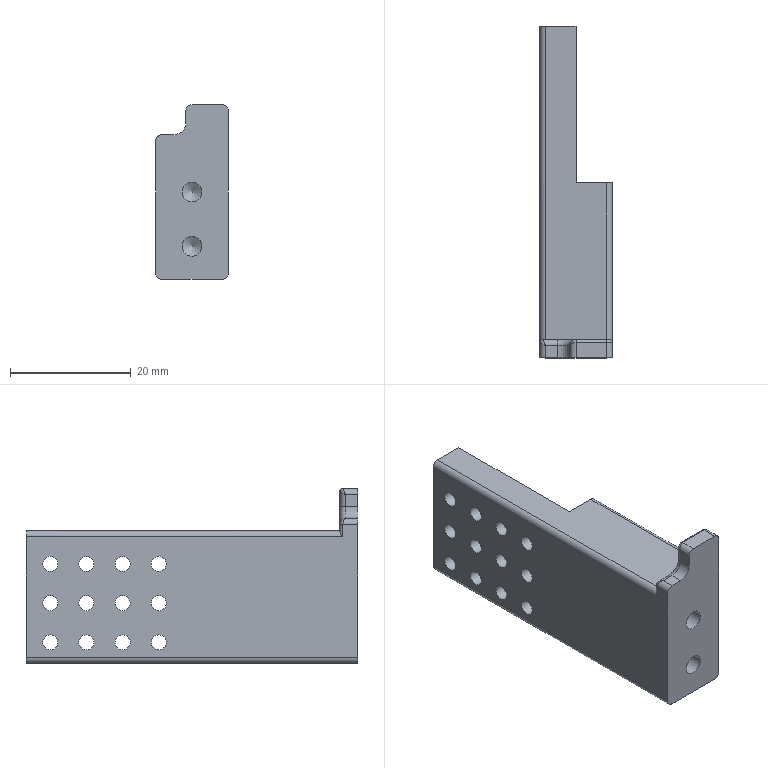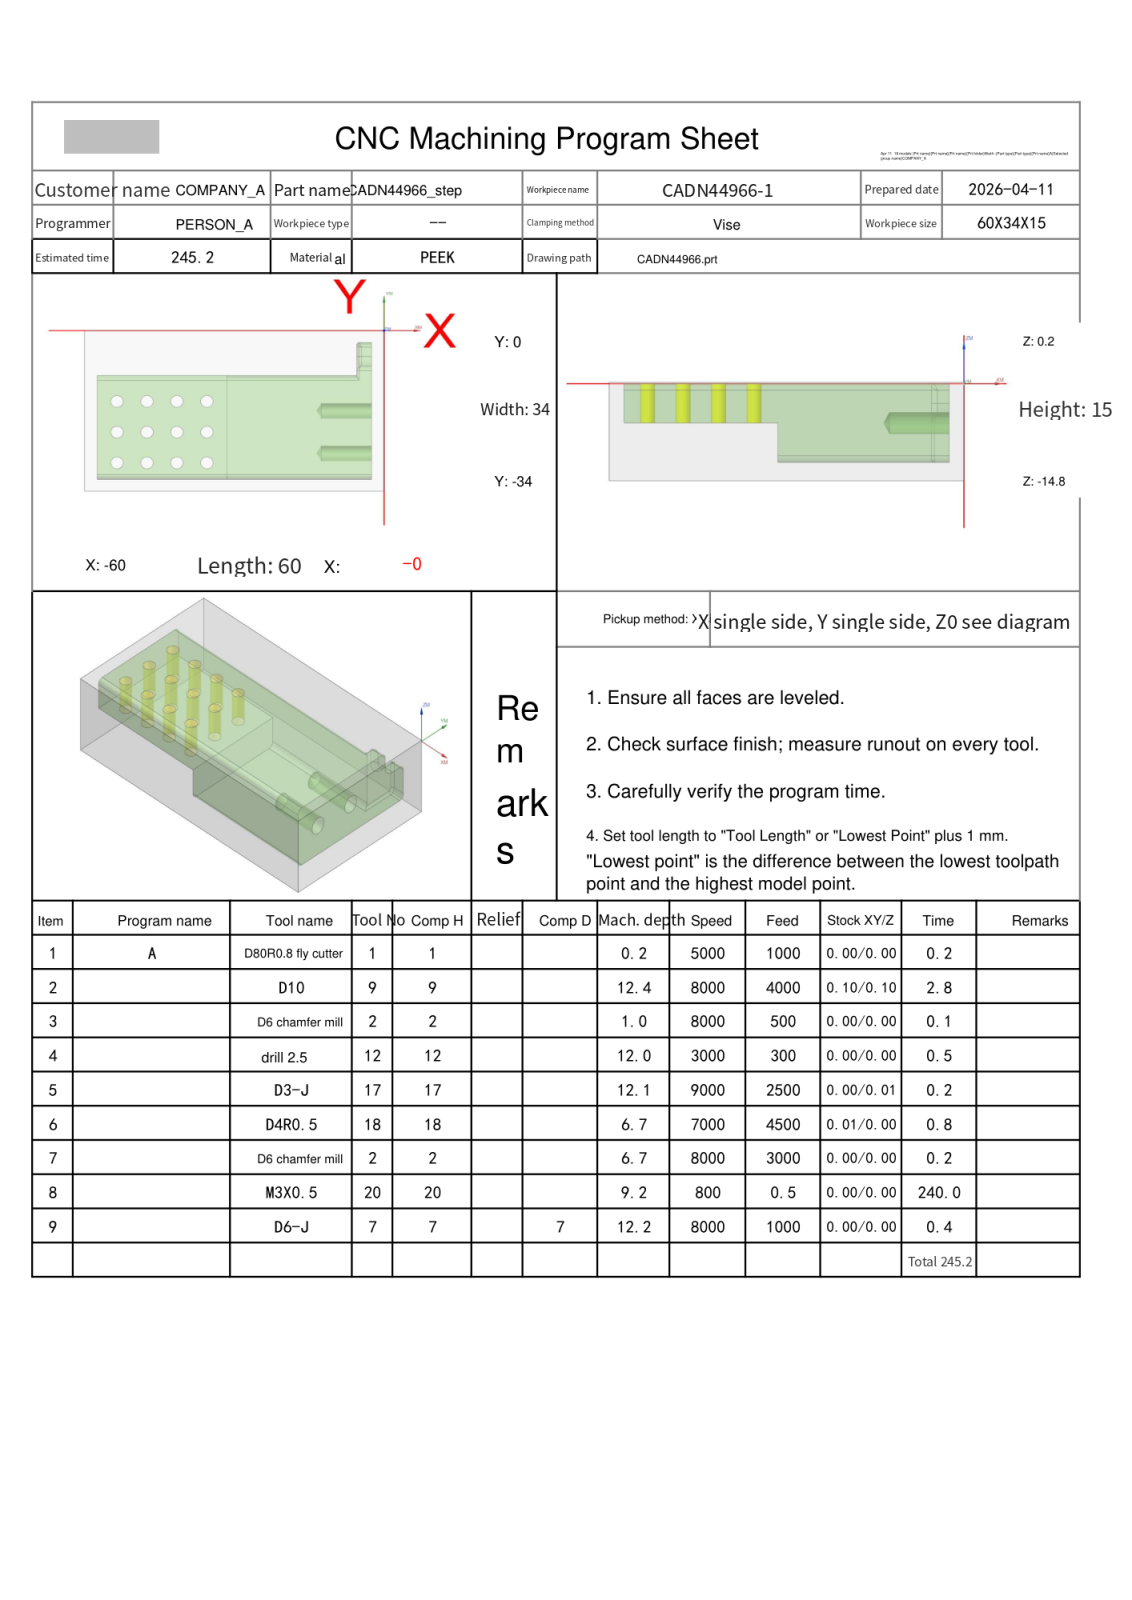NC program | NX | posted by the shop | part box 12 x 55 x 29 mm
Lines 2145 to 3281 of 3281:
N6 T18 M06
(D4R0.5  D=4. R=0.5 H=18 ce=0.01 di=0.00)
G00 G90 G54 X1.72 Y-32.322 M03 S7000
G43 H18 Z10.2
M08
Z.488
G01 Z-.012 F4500.
X-1.4 Y-32.113
G03 X-1.655 Y-32.105 I-.255 J-3.807
X-2.5 Y-32.199 I0.0 J-3.816
G01 X-57.5
X-58.6 Y-32.111
Y-32.156 Z-.02
Y-32.174 Z-.028
X-57.5 Y-32.3
X-2.5
G02 X-1.584 Y-32.179 I.916 J-3.411
G01 X-1.4 Y-32.184
Y-32.251 Z-.038
Y-32.268 Z-.048
X-2.5 Y-32.385
X-57.5
X-58.6 Y-32.25
Y-32.307 Z-.059
Y-32.338 Z-.07
X-57.5 Y-32.463
X-2.5
G02 X-1.42 Y-32.365 I1.08 J-5.877
G01 X-1.4
Y-32.407 Z-.084
Y-32.429 Z-.097
G03 X-2.5 Y-32.541 I.01 J-5.57
G01 X-57.5
G03 X-58.6 Y-32.415 I-1.468 J-7.964
G01 Y-32.465 Z-.113
Y-32.494 Z-.13
G02 X-57.5 Y-32.62 I-.279 J-7.329
G01 X-2.5
G02 X-1.4 Y-32.505 I1.119 J-5.41
G01 Y-32.56 Z-.149
Y-32.595 Z-.168
G03 X-2.5 Y-32.7 I.124 J-7.151
G01 X-57.5
G03 X-58.6 Y-32.588 I-1.463 J-8.959
G01 Y-32.643 Z-.19
Y-32.685 Z-.212
G02 X-57.5 Y-32.779 I-.1 J-7.651
G01 X-2.5
G02 X-1.4 Y-32.688 I1.138 J-7.013
G01 X-1.399 Y-32.734 Z-.237
X-1.398 Y-32.78 Z-.263
X-1.405
G03 X-2.5 Y-32.858 I0.0 J-7.705
G01 X-57.5
G03 X-58.593 Y-32.78 I-1.093 J-7.602
G01 X-58.602
Y-32.818 Z-.291
X-58.601 Y-32.855 Z-.319
X-58.583
G02 X-57.5 Y-32.935 I0.0 J-7.43
G01 X-2.5
G02 X-1.411 Y-32.855 I1.089 J-7.418
G01 X-1.399
X-1.4 Y-32.895 Z-.35
Y-32.934 Z-.38
X-1.45
G03 X-2.5 Y-33.008 I0.0 J-7.494
G01 X-57.5
G03 X-58.547 Y-32.934 I-1.047 J-7.396
G01 X-58.6
X-58.601 Y-32.979 Z-.414
Y-33.012 Z-.447
X-58.596
G02 X-57.5 Y-33.078 I0.0 J-9.139
G01 X-2.5
G02 X-1.401 Y-33.012 I1.099 J-9.111
G01 X-1.399
Y-33.05 Z-.483
Y-33.086 Z-.519
X-1.502 Y-33.085
G03 X-2.5 Y-33.145 I0.0 J-8.383
G01 X-57.5
G03 X-58.494 Y-33.085 I-.994 J-8.274
G01 X-58.602 Y-33.086
X-58.601 Y-33.116 Z-.557
Y-33.145 Z-.596
X-58.517
G02 X-57.5 Y-33.207 I0.0 J-8.403
G01 X-2.5
G02 X-1.48 Y-33.145 I1.02 J-8.367
G01 X-1.399
X-1.4 Y-33.177 Z-.636
Y-33.207 Z-.676
X-1.518
G03 X-2.5 Y-33.264 I0.0 J-8.497
G01 X-57.5
G03 X-58.444 Y-33.206 I-.944 J-7.719
G01 X-58.6 Y-33.208
X-58.601 Y-33.24 Z-.718
X-58.602 Y-33.267 Z-.761
X-58.472 Y-33.266
G02 X-57.5 Y-33.315 I0.0 J-9.699
G01 X-2.5
G02 X-1.52 Y-33.266 I.979 J-9.79
G01 X-1.398 Y-33.267
Y-33.287 Z-.805
Y-33.31 Z-.849
X-1.444
G03 X-2.5 Y-33.361 I0.0 J-10.853
G01 X-57.5
G03 X-58.486 Y-33.312 I-.986 J-9.766
G01 X-58.602
Y-33.335 Z-.894
Y-33.356 Z-.94
X-58.424 Y-33.354
G02 X-57.5 Y-33.401 I0.0 J-9.019
G01 X-2.5
G02 X-1.429 Y-33.35 I1.071 J-11.207
G01 X-1.398
Y-33.371 Z-.987
Y-33.39 Z-1.034
G03 X-2.5 Y-33.436 I.189 J-17.771
G01 X-57.5
G03 X-58.404 Y-33.397 I-.904 J-10.532
G01 X-58.603 Y-33.399
X-58.602 Y-33.415 Z-1.081
Y-33.432 Z-1.129
X-58.426 Y-33.431
G02 X-57.5 Y-33.464 I0.0 J-13.202
G01 X-2.5
G02 X-1.398 Y-33.425 I1.263 J-20.561
G01 X-1.399 Y-33.442 Z-1.176
Y-33.453 Z-1.222
G03 X-2.5 Y-33.484 I.082 J-22.15
G01 X-57.5
G03 X-58.395 Y-33.457 I-.895 J-14.646
X-58.601 Y-33.458 I0.0 J-14.674
G01 X-58.6 Y-33.476 Z-1.268
Y-33.484 Z-1.315
G02 X-58.344 Y-33.483 I.256 J-22.307
X-57.5 Y-33.499 I0.0 J-22.309
G01 X-2.5
X-1.4 Y-33.48
Y-33.491 Z-1.361
Y-33.498 Z-1.407
X-2.5 Y-33.507
X-57.5
X-58.602 Y-33.499
Y-33.508 Z-1.454
X-58.603 Y-33.51 Z-1.5
X-1.4
G00 Z10.2
G00 G90 X-61.837 Y-8.898 M03 S7000
Z10.2
Z.488
G01 Z-.012 F4500.
X-58.603 Y-8.894
X-57.5 Y-8.802
X-6.663
Y-8.5
Y-8.485
G02 X-4.996 Y-6.802 I1.682 J0.0
G01 X-2.5
X-1.4 Y-6.883
Y-6.848 Z-.019
Y-6.83 Z-.026
X-1.411
G02 X-2.5 Y-6.712 I0.0 J5.057
G01 X-4.991
G03 X-6.737 Y-8.479 I.021 J-1.767
G01 Y-8.5
Y-8.712
X-57.5
G02 X-58.316 Y-8.821 I-.816 J2.98
X-58.601 Y-8.808 I0.0 J3.09
G01 X-58.603 Y-8.767 Z-.034
X-58.605 Y-8.726 Z-.043
G03 X-58.274 Y-8.747 I.331 J2.693
X-57.5 Y-8.634 I0.0 J2.714
G01 X-6.8
Y-8.5
Y-8.474
G02 X-4.985 Y-6.634 I1.84 J0.0
G01 X-2.5
X-1.4 Y-6.768
Y-6.71 Z-.054
Y-6.689 Z-.064
X-2.5 Y-6.556
X-4.978
G03 X-6.863 Y-8.47 I.03 J-1.914
G01 X-6.862 Y-8.5
Y-8.556
X-57.5
G02 X-58.43 Y-8.658 I-.93 J4.19
G01 X-58.602 Y-8.655
X-58.601 Y-8.612 Z-.077
X-58.6 Y-8.573 Z-.09
X-58.552 Y-8.574
G03 X-57.5 Y-8.479 I0.0 J5.897
G01 X-6.923
G02 X-4.969 Y-6.479 I2.016 J-.015
G01 X-2.5
X-1.4 Y-6.599
Y-6.56 Z-.105
Y-6.524 Z-.121
G02 X-2.5 Y-6.4 I.299 J7.568
G01 X-4.959
G03 X-6.926 Y-8.015 I.052 J-2.067
G01 X-6.981 Y-8.4
X-57.5
G02 X-58.6 Y-8.505 I-1.107 J5.765
G01 Y-8.46 Z-.139
Y-8.424 Z-.158
G03 X-57.5 Y-8.32 I-.041 J6.28
G01 X-7.038
G02 X-4.947 Y-6.32 I2.144 J-.149
G01 X-2.5
G03 X-1.4 Y-6.435 I1.366 J7.711
G01 Y-6.382 Z-.18
Y-6.332 Z-.201
G02 X-2.5 Y-6.24 I.09 J7.674
G01 X-4.933
G03 X-7.092 Y-8.24 I.063 J-2.233
G01 X-57.5
G02 X-58.6 Y-8.33 I-1.264 J8.632
G01 Y-8.284 Z-.225
Y-8.25 Z-.25
G03 X-57.5 Y-8.161 I-.001 J6.861
G01 X-7.142
G02 X-4.916 Y-6.161 I2.28 J-.299
G01 X-2.5
G03 X-1.399 Y-6.249 I1.165 J7.674
G01 Y-6.202 Z-.277
Y-6.163 Z-.305
X-1.434 Y-6.164
G02 X-2.5 Y-6.084 I0.0 J7.173
G01 X-4.898
G03 X-7.184 Y-8.073 I.051 J-2.366
G01 X-7.201 Y-8.084
X-57.5
G02 X-58.6 Y-8.174 I-1.183 J7.718
G01 Y-8.124 Z-.335
Y-8.09 Z-.365
G03 X-57.5 Y-8.01 I-.047 J8.233
G01 X-7.231
G02 X-4.878 Y-6.01 I2.407 J-.448
G01 X-2.5
G03 X-1.4 Y-6.085 I1.142 J8.595
G01 Y-6.042 Z-.398
X-1.399 Y-6.001 Z-.43
X-1.432
G02 X-2.5 Y-5.938 I0.0 J9.084
G01 X-4.856
G03 X-7.265 Y-7.938 I.05 J-2.511
G01 X-57.5
G02 X-58.536 Y-8.002 I-1.036 J8.448
G01 X-58.6 Y-8.001
X-58.601 Y-7.96 Z-.466
Y-7.929 Z-.501
X-58.519
G03 X-57.5 Y-7.871 I0.0 J8.943
G01 X-7.296
G02 X-5.641 Y-6.012 I2.54 J-.596
X-4.833 Y-5.871 I.808 J-2.242
G01 X-2.5
G03 X-1.461 Y-5.931 I1.039 J8.991
G01 X-1.399
Y-5.899 Z-.539
Y-5.869 Z-.576
X-1.505 Y-5.87
G02 X-2.5 Y-5.808 I0.0 J8.056
G01 X-4.808
G03 X-7.321 Y-7.81 I.047 J-2.637
G01 X-7.333 Y-7.808
X-57.5
G02 X-58.492 Y-7.87 I-.992 J7.94
G01 X-58.601 Y-7.869
Y-7.838 Z-.616
Y-7.809 Z-.656
X-58.502 Y-7.81
G03 X-57.5 Y-7.75 I0.0 J8.419
G01 X-7.347
G02 X-5.68 Y-5.915 I2.647 J-.73
X-4.781 Y-5.75 I.999 J-2.915
G01 X-2.5
G03 X-1.4 Y-5.808 I1.131 J10.987
G01 Y-5.775 Z-.698
Y-5.75 Z-.74
X-1.445
G02 X-2.5 Y-5.697 I0.0 J10.496
G01 X-4.753
X-4.802 Y-5.704
X-5.085 Y-5.72
G03 X-7.357 Y-7.697 I.382 J-2.734
G01 X-57.5
G02 X-58.519 Y-7.747 I-1.019 J10.41
G01 X-58.6 Y-7.746
Y-7.725 Z-.783
Y-7.701 Z-.827
X-58.462 Y-7.702
G03 X-57.5 Y-7.649 I0.0 J8.811
G01 X-7.367
G02 X-6.217 Y-6.104 I2.749 J-.845
X-4.724 Y-5.649 I1.543 J-2.386
G01 X-2.5
G03 X-1.4 Y-5.705 I1.116 J11.228
G01 Y-5.676 Z-.872
Y-5.658 Z-.917
X-1.453
G02 X-2.5 Y-5.608 I0.0 J10.934
G01 X-4.694
G03 X-7.367 Y-7.608 I.039 J-2.838
G01 X-57.5
G02 X-58.589 Y-7.661 I-1.089 J11.136
G01 X-58.6
Y-7.639 Z-.964
Y-7.619 Z-1.011
G03 X-57.5 Y-7.572 I-.112 J15.527
G01 X-7.364
G02 X-4.663 Y-5.572 I2.742 J-.879
G01 X-2.5
G03 X-1.584 Y-5.615 I.916 J9.853
G01 X-1.4 Y-5.613
X-1.399 Y-5.59 Z-1.058
X-1.398 Y-5.576 Z-1.106
X-1.578 Y-5.578
G02 X-2.5 Y-5.543 I0.0 J12.213
G01 X-4.631
G03 X-7.354 Y-7.543 I.039 J-2.907
G01 X-57.5
G02 X-58.599 Y-7.581 I-1.206 J18.777
G01 X-58.6 Y-7.564 Z-1.155
Y-7.548 Z-1.203
G03 X-57.5 Y-7.52 I-.149 J26.922
G01 X-7.346
G02 X-4.599 Y-5.52 I2.789 J-.945
G01 X-2.5
G03 X-1.615 Y-5.545 I.885 J15.399
X-1.396 Y-5.544 I0.0 J15.425
G01 X-1.395 Y-5.535 Z-1.253
X-1.394 Y-5.519 Z-1.302
G02 X-1.646 Y-5.521 I-.252 J20.394
X-2.5 Y-5.503 I0.0 J20.395
G01 X-4.566
X-4.607 Y-5.51
G03 X-5.753 Y-5.763 I.025 J-2.833
X-7.339 Y-7.503 I1.264 J-2.745
G01 X-57.5
G02 X-58.601 Y-7.523 I-1.11 J30.954
G01 X-58.602 Y-7.515 Z-1.352
Y-7.505 Z-1.401
X-57.5 Y-7.493
X-7.335
G02 X-4.677 Y-5.493 I2.841 J-1.009
G01 X-2.5
G03 X-1.649 Y-5.504 I.851 J33.099
G01 X-1.395 Y-5.503
Y-5.494 Z-1.451
Y-5.491 Z-1.5
X-2.5 Y-5.49
X-4.646
G03 X-7.335 Y-7.49 I.158 J-3.021
G01 X-7.491
X-57.5
X-58.603
G00 Z10.2
G00 G90 X-8.666 Y-6.802 M03 S7000
Z10.2
Z.488
G01 Z-.012 F4500.
G03 X-6.666 Y-8.802 I2. J0.0
G01 X-6.675 Y-8.619
G02 X-4.996 Y-6.802 I1.822 J0.0
G01 X-2.5
X-1.399 Y-6.901
Y-6.848 Z-.019
Y-6.826 Z-.026
X-1.526 Y-6.828
G02 X-2.5 Y-6.712 I0.0 J4.152
G01 X-4.991
G03 X-6.747 Y-8.545 I.079 J-1.833
G01 X-6.739 Y-8.712
X-6.757
Y-8.683 Z-.032
X-6.768 Y-8.657 Z-.037
X-6.803 Y-8.633 Z-.043
X-6.806 Y-8.522
G02 X-4.985 Y-6.633 I1.89 J0.0
G01 X-2.5
G03 X-1.399 Y-6.764 I1.139 J4.875
G01 Y-6.712 Z-.054
Y-6.691 Z-.064
G02 X-2.5 Y-6.555 I.5 J8.593
G01 X-4.978
G03 X-6.866 Y-8.519 I.077 J-1.963
G01 Y-8.555
X-6.881
X-6.885 Y-8.523 Z-.073
X-6.892 Y-8.501 Z-.082
X-6.928 Y-8.477 Z-.091
G02 X-4.969 Y-6.477 I2.023 J-.022
G01 X-2.5
G03 X-1.4 Y-6.602 I1.619 J9.345
G01 Y-6.56 Z-.106
Y-6.519 Z-.122
G02 X-2.5 Y-6.397 I.201 J6.798
G01 X-4.959
G03 X-6.985 Y-8.397 I.064 J-2.091
G01 X-6.999
X-6.998 Y-8.368 Z-.135
X-7.021 Y-8.331 Z-.148
X-7.042 Y-8.315 Z-.16
G02 X-4.946 Y-6.315 I2.164 J-.169
G01 X-2.5
G03 X-1.4 Y-6.43 I1.188 J6.081
G01 Y-6.377 Z-.182
Y-6.326 Z-.204
X-1.439
G02 X-2.5 Y-6.235 I0.0 J6.189
G01 X-4.932
G03 X-7.095 Y-8.235 I.056 J-2.23
G01 X-7.146 Y-8.156 Z-.254
G02 X-4.915 Y-6.156 I2.304 J-.325
G01 X-2.5
G02 X-1.924 Y-6.244 I-.064 J-2.338
G01 X-1.4 Y-6.245
Y-6.196 Z-.281
Y-6.168 Z-.309
X-1.924 Y-6.167
G03 X-2.5 Y-6.078 I-.671 J-2.44
G01 X-4.897
G03 X-7.186 Y-8.066 I.049 J-2.368
G01 X-7.203 Y-8.078
X-7.233 Y-8.004 Z-.37
G02 X-4.877 Y-6.004 I2.415 J-.457
G01 X-2.5
G02 X-1.924 Y-6.082 I-.122 J-3.048
G01 X-1.4 Y-6.083
Y-6.036 Z-.403
Y-5.996 Z-.436
X-1.573 Y-5.998
G02 X-2.5 Y-5.933 I0.0 J6.632
G01 X-4.855
G03 X-7.268 Y-7.933 I.048 J-2.513
G01 X-7.299 Y-7.866 Z-.507
G02 X-4.831 Y-5.866 I2.517 J-.583
G01 X-2.5
G03 X-1.561 Y-5.926 I.938 J7.256
G01 X-1.4 Y-5.924
Y-5.894 Z-.545
Y-5.865 Z-.583
X-1.576 Y-5.867
G02 X-2.5 Y-5.803 I0.0 J6.74
G01 X-4.806
G03 X-5.81 Y-6.017 I.083 J-2.859
X-7.327 Y-7.803 I1.093 J-2.464
G01 X-7.343 Y-7.745 Z-.663
G02 X-4.779 Y-5.745 I2.607 J-.699
G01 X-2.5
G03 X-1.574 Y-5.806 I.926 J7.011
G01 X-1.4 Y-5.804
Y-5.773 Z-.705
Y-5.741 Z-.747
X-1.579 Y-5.743
G02 X-2.5 Y-5.693 I0.0 J8.504
G01 X-4.751
G03 X-7.358 Y-7.693 I.043 J-2.755
G01 X-7.366 Y-7.646 Z-.834
G02 X-4.721 Y-5.646 I2.686 J-.803
G01 X-2.5
X-1.924 Y-5.697
X-1.4
X-1.401 Y-5.672 Z-.88
Y-5.653 Z-.925
G02 X-1.623 Y-5.656 I-.222 J7.508
X-2.5 Y-5.605 I0.0 J7.511
G01 X-4.692
G03 X-7.004 Y-6.86 I.031 J-2.814
X-7.365 Y-7.605 I2.346 J-1.596
G01 X-7.385 Y-7.569 Z-1.018
X-7.359 Y-7.559
X-7.332 Y-7.482
G02 X-4.66 Y-5.569 I2.711 J-.966
G01 X-2.5
G03 X-1.662 Y-5.612 I.838 J8.316
X-1.402 Y-5.607 I0.0 J8.359
G01 Y-5.59 Z-1.066
Y-5.572 Z-1.114
G02 X-1.711 Y-5.578 I-.309 J8.411
X-2.5 Y-5.541 I0.0 J8.416
G01 X-4.629
X-4.815 Y-5.553
G03 X-6.774 Y-6.528 I.191 J-2.839
X-7.353 Y-7.541 I2.274 J-1.972
G01 X-7.345 Y-7.518 Z-1.211
G02 X-6.253 Y-6.053 I2.845 J-.982
X-4.63 Y-5.524 I1.657 J-2.327
G01 X-4.596 Y-5.518
X-2.5
G03 X-1.726 Y-5.546 I.774 J10.621
X-1.402 Y-5.541 I0.0 J10.65
G01 X-1.4 Y-5.525 Z-1.261
X-1.399 Y-5.521 Z-1.31
G02 X-1.613 Y-5.522 I-.214 J19.642
X-2.5 Y-5.502 I0.0 J19.643
G01 X-4.563
G03 X-5.644 Y-5.716 I.031 J-2.992
X-7.34 Y-7.502 I1.144 J-2.784
G01 X-7.336 Y-7.493 Z-1.41
G02 X-4.628 Y-5.493 I2.836 J-1.007
G01 X-2.5
X-2.484 Y-5.496
X-1.401 Y-5.502
X-1.399 Y-5.492 Z-1.459
Z-1.509
X-2.5 Y-5.49
X-4.5
G03 X-7.335 Y-7.49 I0.0 J-3.01
G01 Z-1.609
G02 X-4.5 Y-5.49 I2.835 J-1.01
G01 X-2.5
X-1.399 Y-5.491
Z-1.709
X-2.5 Y-5.49
X-4.5
G03 X-7.335 Y-7.49 I0.0 J-3.01
G01 Z-1.809
G02 X-4.5 Y-5.49 I2.835 J-1.01
G01 X-2.5
X-1.399 Y-5.491
X-1.4 Z-1.909
X-2.5 Y-5.49
X-4.5
G03 X-7.335 Y-7.49 I0.0 J-3.01
G01 Z-2.009
G02 X-4.5 Y-5.49 I2.835 J-1.01
G01 X-2.5
X-1.4 Y-5.491
Z-2.109
X-2.5 Y-5.49
X-4.5
G03 X-7.335 Y-7.49 I0.0 J-3.01
G01 Z-2.209
G02 X-4.5 Y-5.49 I2.835 J-1.01
G01 X-2.5
X-1.4 Y-5.491
Z-2.309
X-2.5 Y-5.49
X-4.5
G03 X-7.335 Y-7.49 I0.0 J-3.01
G01 Z-2.409
G02 X-4.5 Y-5.49 I2.835 J-1.01
G01 X-2.5
X-1.4 Y-5.491
Z-2.509
X-2.5 Y-5.49
X-4.5
G03 X-7.335 Y-7.49 I0.0 J-3.01
G01 Z-2.609
G02 X-4.5 Y-5.49 I2.835 J-1.01
G01 X-2.5
X-1.4 Y-5.491
Z-2.709
X-2.5 Y-5.49
X-4.5
G03 X-7.335 Y-7.49 I0.0 J-3.01
G01 Z-2.809
G02 X-4.5 Y-5.49 I2.835 J-1.01
G01 X-2.5
X-1.4 Y-5.491
Y-5.49 Z-2.909
X-2.5
X-4.5
G03 X-7.335 Y-7.49 I0.0 J-3.01
G01 Z-3.009
G02 X-4.5 Y-5.49 I2.835 J-1.01
G01 X-2.5
X-1.4
Z-3.109
X-2.5
X-4.5
G03 X-7.335 Y-7.49 I0.0 J-3.01
G01 Z-3.209
G02 X-4.5 Y-5.49 I2.835 J-1.01
G01 X-2.5
X-1.4
Z-3.309
X-2.5
X-4.5
G03 X-7.335 Y-7.49 I0.0 J-3.01
G01 Z-3.409
G02 X-4.5 Y-5.49 I2.835 J-1.01
G01 X-2.5
X-1.4
Y-5.482 Z-3.509
X-2.536 Y-5.49
X-4.504
X-4.63 Y-5.493
G03 X-7.335 Y-7.49 I.13 J-3.007
G01 Z-3.609
G02 X-6.692 Y-6.437 I2.835 J-1.01
X-4.5 Y-5.486 I2.197 J-2.061
G01 X-2.5
X-2.484 Y-5.483
X-1.4 Y-5.463
Y-5.449 Z-3.658
Y-5.439 Z-3.708
X-2.204 Y-5.453
X-2.255 Y-5.455
X-2.484 Y-5.468
X-2.5 Y-5.476
X-4.5
X-4.531 Y-5.473
X-4.808 Y-5.493
G03 X-6.74 Y-6.48 I.275 J-2.922
X-7.337 Y-7.49 I2.135 J-1.943
G01 X-7.343 Z-3.806
G02 X-6.867 Y-6.618 I2.683 J-.901
X-5.762 Y-5.736 I2.317 J-1.768
X-4.512 Y-5.458 I1.249 J-2.672
G01 X-4.5
X-2.6
X-2.573 Y-5.452
X-2.204 Y-5.423
X-1.4 Y-5.412
Y-5.398 Z-3.854
Y-5.384 Z-3.903
X-2.204 Y-5.392
X-2.231
G03 X-2.635 Y-5.435 I0.0 J-1.914
G01 X-4.521
G03 X-5.663 Y-5.669 I0.0 J-2.903
X-7.35 Y-7.49 I1.201 J-2.804
G01 X-7.356 Z-3.998
G02 X-5.564 Y-5.601 I2.927 J-.983
X-4.534 Y-5.405 I1.031 J-2.607
G01 X-2.649
G02 X-2.229 Y-5.356 I.42 J-1.78
G01 X-2.204
X-1.4 Y-5.351
Y-5.34 Z-4.044
Y-5.318 Z-4.09
X-2.33 Y-5.32
G03 X-2.653 Y-5.369 I.002 J-1.104
G01 X-4.537
G03 X-5.564 Y-5.567 I0.0 J-2.76
X-7.361 Y-7.49 I1.156 J-2.881
G01 X-7.368 Z-4.18
G02 X-5.697 Y-5.585 I2.992 J-.939
X-4.504 Y-5.327 I1.193 J-2.631
G01 X-4.5
X-2.687
G02 X-2.214 Y-5.27 I.473 J-1.918
G01 X-2.204
X-1.4 Y-5.268
Y-5.248 Z-4.223
Y-5.219 Z-4.266
X-2.204
G03 X-2.684 Y-5.279 I.022 J-2.116
G01 X-4.5
G03 X-5.284 Y-5.383 I.002 J-3.034
X-7.374 Y-7.49 I.932 J-3.014
G01 X-7.38 Z-4.349
G02 X-5.729 Y-5.508 I3.061 J-.871
X-4.528 Y-5.226 I1.201 J-2.422
G01 X-4.5
X-2.5
G02 X-2.204 Y-5.17 I.304 J-.785
G01 X-1.4
Y-5.137 Z-4.389
Y-5.105 Z-4.428
X-2.204
X-2.236
G03 X-2.726 Y-5.168 I0.0 J-1.913
G01 X-4.5
X-4.517
G03 X-5.746 Y-5.465 I0.0 J-2.7
X-7.386 Y-7.49 I1.463 J-2.861
G01 X-7.397 Z-4.502
G02 X-5.844 Y-5.463 I3.192 J-.836
X-4.5 Y-5.106 I1.346 J-2.36
G01 X-2.5
X-2.204 Y-5.044
X-1.4
Y-5.004 Z-4.537
Y-4.968 Z-4.572
X-2.204 Y-4.967
X-2.5 Y-5.04
X-4.502
G03 X-5.678 Y-5.32 I0.0 J-2.602
X-7.403 Y-7.49 I1.503 J-2.967
G01 X-7.412 Z-4.636
G02 X-5.844 Y-5.342 I3.366 J-.811
X-4.5 Y-4.969 I1.36 J-2.293
G01 X-2.746
G02 X-2.245 Y-4.892 I.501 J-1.574
G01 X-2.204
X-1.4
Y-4.856 Z-4.666
Y-4.811 Z-4.695
X-2.285
G03 X-2.738 Y-4.896 I0.0 J-1.244
G01 X-4.5
G03 X-5.797 Y-5.256 I0.0 J-2.518
X-7.42 Y-7.49 I1.82 J-3.028
G01 X-7.426 Z-4.749
G02 X-5.805 Y-5.196 I3.554 J-.792
X-4.501 Y-4.821 I1.305 J-2.083
G01 X-2.5
X-2.204 Y-4.732
X-1.924
X-1.4
Y-4.687 Z-4.772
Y-4.643 Z-4.796
G03 X-1.796 Y-4.624 I-.396 J-4.242
X-2.804 Y-4.745 I0.0 J-4.26
G01 X-4.5
G03 X-5.844 Y-5.156 I.03 J-2.501
X-7.432 Y-7.49 I2.096 J-3.132
G01 X-7.438 Z-4.838
G02 X-5.785 Y-5.056 I3.81 J-.81
X-4.502 Y-4.669 I1.283 J-1.929
G01 X-2.798
G02 X-1.743 Y-4.533 I1.056 J-4.016
X-1.4 Y-4.547 I0.0 J-4.153
G01 Y-4.524 Z-4.855
Y-4.455 Z-4.873
X-1.924 Y-4.476
X-2.204 Y-4.461
X-2.259 Y-4.459
G03 X-2.806 Y-4.594 I0.0 J-1.175
G01 X-4.5
G03 X-5.844 Y-5.041 I.026 J-2.325
X-7.442 Y-7.49 I2.327 J-3.264
G01 X-7.446 Z-4.902
G02 X-5.671 Y-4.868 I4.051 J-.83
X-4.523 Y-4.523 I1.148 J-1.741
G01 X-2.87
G02 X-1.761 Y-4.362 I1.109 J-3.741
X-1.4 Y-4.379 I0.0 J-3.902
G01 Y-4.35 Z-4.914
Y-4.311 Z-4.926
G03 X-1.764 Y-4.294 I-.364 J-3.825
X-2.87 Y-4.456 I0.0 J-3.843
G01 X-4.516
G03 X-5.665 Y-4.81 I0.0 J-2.041
X-7.449 Y-7.49 I2.406 J-3.535
G01 X-7.451 Z-4.945
G02 X-6.685 Y-5.769 I4.119 J-.804
X-5.681 Y-4.768 I3.516 J-2.523
X-4.503 Y-4.391 I1.178 J-1.652
G01 X-2.84
G02 X-1.74 Y-4.219 I1.1 J-3.43
X-1.402 Y-4.235 I0.0 J-3.602
G01 Y-4.227 Z-4.953
X-1.403 Y-4.176 Z-4.961
G03 X-1.73 Y-4.16 I-.327 J-3.437
X-2.803 Y-4.331 I0.0 J-3.453
G01 X-4.5
X-4.533
G03 X-5.504 Y-4.612 I0.0 J-1.813
X-6.672 Y-5.736 I2.159 J-3.413
X-7.453 Y-7.49 I3.377 J-2.554
G01 X-7.455 Z-4.975
G02 X-6.685 Y-5.734 I4.219 J-.804
X-5.623 Y-4.633 I3.852 J-2.651
X-4.503 Y-4.262 I1.12 J-1.506
G01 X-2.812
G02 X-1.765 Y-4.101 I1.047 J-3.327
X-1.404 Y-4.12 I0.0 J-3.488
G01 X-1.414 Y-4.08 Z-4.985
G03 X-1.882 Y-4.034 I-.468 J-2.375
X-2.764 Y-4.201 I0.0 J-2.421
G01 X-4.5
X-4.516
G03 X-5.564 Y-4.552 I0.0 J-1.741
X-6.695 Y-5.736 I2.927 J-3.926
X-7.456 Y-7.49 I3.505 J-2.562
G01 X-7.457 Z-5.
G02 X-6.685 Y-5.705 I4.368 J-.83
X-5.749 Y-4.627 I6.816 J-4.973
G03 X-5.419 Y-4.397 I-8.528 J12.601
G02 X-4.699 Y-4.12 I.72 J-.797
G01 X-4.645 Y-4.122
X-4.5 Y-4.112
X-2.831
X-2.507 Y-4.016
G00 Z10.2
G00 G90 X-8.166 Y-4.323 M03 S7000
Z10.2
Z-4.508
G01 Z-5.008 F4500.
X-6.166 Y-5.011
Y-3.448
G02 X-4.543 Y-1.834 I1.623 J-.009
G01 X-4.534
X-2.5
G03 X-1.662 Y-1.938 I.838 J3.325
X-1.399 Y-1.928 I0.0 J3.429
G01 X-1.4 Y-1.865 Z-5.015
Y-1.859 Z-5.022
X-1.549 Y-1.862
G02 X-2.5 Y-1.732 I0.0 J3.542
G01 X-4.576
X-4.579
G03 X-6.268 Y-3.418 I0.0 J-1.689
G01 Y-5.1
X-6.356 Y-5.165 Z-5.04
Y-3.385
G02 X-4.615 Y-1.644 I1.741 J0.0
G01 X-2.5
G03 X-1.4 Y-1.771 I8.58 J69.579
G01 Y-1.712 Z-5.051
Y-1.673 Z-5.062
G02 X-2.5 Y-1.564 I.136 J6.984
G01 X-4.642
G03 X-6.436 Y-3.358 I0.0 J-1.794
G01 Y-5.237
X-6.516 Y-5.293 Z-5.088
Y-3.332
G02 X-4.668 Y-1.484 I1.848 J0.0
G01 X-2.5
G03 X-1.399 Y-1.597 I1.2 J6.273
G01 Y-1.555 Z-5.104
Y-1.514 Z-5.119
G02 X-2.5 Y-1.404 I.034 J5.881
G01 X-4.695
G03 X-6.596 Y-3.305 I0.0 J-1.901
G01 Y-5.334
X-6.677 Y-5.377 Z-5.156
Y-3.278
G02 X-4.722 Y-1.323 I1.955 J0.0
G01 X-2.5
G03 X-1.4 Y-1.432 I1.241 J6.918
G01 Y-1.385 Z-5.178
Y-1.34 Z-5.199
G02 X-2.5 Y-1.244 I.029 J6.67
G01 X-4.749
G03 X-6.756 Y-3.251 I0.0 J-2.008
G01 Y-5.357
X-6.835 Y-5.451 Z-5.247
Y-3.226
G02 X-4.774 Y-1.165 I2.061 J0.0
G01 X-2.5
G03 X-1.545 Y-1.245 I.955 J5.632
G01 X-1.4 Y-1.244
Y-1.206 Z-5.274
Y-1.17 Z-5.301
X-1.95
G03 X-2.5 Y-1.089 I-.596 J-2.144
G01 X-4.8
G03 X-6.911 Y-3.2 I0.0 J-2.111
G01 Y-5.5
X-6.995 Y-5.566 Z-5.359
X-6.984 Y-5.5
Y-3.176
G02 X-4.824 Y-1.016 I2.16 J0.0
G01 X-2.5
G02 X-1.95 Y-1.093 I-.124 J-2.908
G01 X-1.4
Y-1.051 Z-5.391
Y-1.012 Z-5.422
X-1.95
G03 X-2.5 Y-.947 I-.746 J-3.941
G01 X-4.848
G03 X-7.053 Y-3.152 I0.0 J-2.206
G01 Y-5.5
X-7.072 Y-5.638
X-7.144 Y-5.72 Z-5.49
X-7.119 Y-5.5
Y-3.13
G02 X-4.87 Y-.881 I2.25 J0.0
G01 X-2.5
G03 X-1.586 Y-.945 I.914 J6.438
G01 X-1.4 Y-.943
Y-.91 Z-5.527
Y-.883 Z-5.563
X-1.95
G03 X-2.5 Y-.819 I-.81 J-4.573
G01 X-4.89
G03 X-7.181 Y-3.11 I0.0 J-2.291
G01 Y-5.5
X-7.177 Y-5.546
X-7.216 Y-5.819
X-7.284 Y-5.942 Z-5.64
G03 X-7.239 Y-5.558 I-1.601 J.384
G01 Y-3.091
G02 X-4.909 Y-.761 I2.335 J-.005
G01 X-2.5
G03 X-1.596 Y-.823 I.904 J6.576
G01 X-1.4 Y-.82
Y-.79 Z-5.68
Y-.759 Z-5.721
G02 X-1.611 Y-.762 I-.211 J7.352
X-2.5 Y-.708 I0.0 J7.355
G01 X-4.927
G03 X-7.292 Y-3.073 I.004 J-2.369
G01 Y-5.5
G02 X-7.347 Y-6.065 I-3.083 J.017
G01 X-7.397 Y-6.171 Z-5.806
G03 X-7.34 Y-5.5 I-3.936 J.674
G01 Y-3.058
G02 X-6.348 Y-1.116 I2.415 J-.009
X-4.942 Y-.66 I1.43 J-2.017
G01 X-2.5
X-1.95 Y-.71
X-1.4
Y-.686 Z-5.85
Y-.664 Z-5.894
X-1.95 Y-.665
X-2.5 Y-.618
X-4.957
G03 X-6.741 Y-1.399 I.015 J-2.462
X-7.382 Y-3.043 I1.862 J-1.673
G01 Y-5.5
G02 X-7.438 Y-6.312 I-6.645 J.049
G01 X-7.46 Y-6.393 Z-5.94
X-7.477 Y-6.474 Z-5.986
G03 X-7.419 Y-5.5 I-10.064 J1.091
G01 Y-3.031
G02 X-4.969 Y-.581 I2.45 J0.0
G01 X-2.5
G03 X-1.673 Y-.625 I.827 J7.814
X-1.4 Y-.62 I0.0 J7.857
G01 Y-.6 Z-6.033
Y-.584 Z-6.08
G02 X-1.695 Y-.589 I-.295 J8.364
X-2.5 Y-.55 I0.0 J8.369
G01 X-4.979
G03 X-7.45 Y-3.021 I.007 J-2.478
G01 Y-5.5
G02 X-7.498 Y-6.603 I-14.465 J.074
G01 X-7.504 Z-6.176
X-7.474 Y-5.64
X-7.475 Y-5.5
Y-3.012
G02 X-4.988 Y-.525 I2.487 J0.0
G01 X-2.5
G03 X-1.729 Y-.553 I.771 J10.87
X-1.402 Y-.548 I0.0 J10.897
G01 X-1.418 Y-.526 Z-6.257
G02 X-1.807 Y-.534 I-.389 J10.126
X-2.5 Y-.51 I0.0 J10.134
G01 X-4.993
G03 X-5.925 Y-.692 I.056 J-2.765
X-7.49 Y-3.007 I.952 J-2.33
G01 Y-5.5
X-7.488 Y-5.64
X-7.508 Y-6.603
X-7.51 Y-6.612 Z-6.338
X-7.496 Y-5.64
X-7.501 Y-5.5
Y-3.003
G02 X-5.961 Y-.692 I2.531 J-.018
X-4.997 Y-.499 I1.032 J-2.649
G01 X-2.5
G03 X-1.809 Y-.517 I.691 J12.917
X-1.433 Y-.512 I0.0 J12.936
G01 X-1.448 Y-.499 Z-6.419
X-2.5 Y-.492
X-4.999
G03 X-7.508 Y-3.001 I.01 J-2.519
G01 Y-5.5
X-7.51 Y-6.612
Z-6.5
Y-3.
G02 X-5.007 Y-.491 I2.51 J-.001
G01 X-1.668 Y-.492
X-1.463 Y-.49
G00 Z10.2
G91 G28 Z0.0
M05
M09
G91 G28 Z0.0
M01
N7 T02 M06
(D6 chamfer mill  D=6. R=0. H=02 ce=0.00 di=0.00)
G00 G90 G54 X-59.628 Y-30.75 M03 S8000
G43 H02 Z20.
M08
Z2.085
G01 Z-1.499 F3000.
G03 X-59.328 Y-30.83 I.3 J.52
X-58.808 Y-30.53 I0.0 J.6
G01 X-58.8 Y-30.5
Y-10.5
X-58.808 Y-10.47
G03 X-59.328 Y-10.17 I-.52 J-.3
X-59.628 Y-10.25 I0.0 J-.6
G01 Z2.085
G00 Z20.
X-.372 Y-8.25
Z2.085
G01 Z-1.499
G03 X-.672 Y-8.17 I-.3 J-.52
X-1.192 Y-8.47 I0.0 J-.6
G01 X-1.2 Y-8.5
Y-30.5
X-1.192 Y-30.53
G03 X-.672 Y-30.83 I.52 J.3
X-.372 Y-30.75 I0.0 J.6
G01 Z2.085
G00 Z20.
Y-3.25
Z-.177
G01 Z-6.499
G03 X-.672 Y-3.17 I-.3 J-.52
X-1.192 Y-3.47 I0.0 J-.6
G01 X-1.2 Y-3.5
Y-4.219
X-1.192 Y-4.249
G03 X-.672 Y-4.549 I.52 J.3
X-.372 Y-4.468 I0.0 J.6
G01 Z1.669
G00 Z20.
G00 G90 X-53.5 Y-15. M03 S8000
Z20.
G98 G81 X-53.5 Y-15. Z-1.75 R3. F500.
X-47.5
X-41.5
X-35.5
Y-21.5
X-41.5
X-47.5
X-53.5
Y-28.
X-47.5
X-41.5
X-35.5
G80
G00 Z20.
G91 G28 Z0.0
M05
M09
G91 G28 Z0.0
M01
N8 T20 M06
(M3X0.5 D=2.5 DR_a=180 H=20)
G00 G90 G54 X-53.5 Y-15. M03 S800
G43 H20 Z20.
M08
G95
G98 G84 X-53.5 Y-15. Z-9. R1. F.5 Q5.
X-47.5
X-41.5
X-35.5
Y-21.5
X-41.5
X-47.5
X-53.5
Y-28.
X-47.5
X-41.5
X-35.5
G80
G94
G00 Z20.
G91 G28 Z0.0
M05
M09
G91 G28 Z0.0
M01
N9 T07 M06
(D6-J  D=6. R=0. H=07 ce=0.00 di=0.00)
G00 G90 G54 X-1.583 Y-35.495 M03 S8000
G43 H07 Z5.2
M08
Z-5.
G01 Z-6. F1000.
G41 D07
X-1.606 Y-35.296
G03 X-2.5 Y-34.5 I-.894 J-.104
G01 X-57.5
G02 X-60.5 Y-31.5 I0.0 J3.
G01 Y-9.5
G02 X-57.5 Y-6.5 I3. J0.0
G01 X-8.5
Y-5.673
X-8.499 Y-2.927
G02 X-5. Y.5 I3.501 J-.075
G01 X-2.5
G02 X.5 Y-2.5 I0.0 J-3.
G01 Y-31.5
G02 X-2.5 Y-34.5 I-3. J0.0
G03 X-3.4 Y-35.4 I0.0 J-.9
G01 G40 Y-35.6
Z-5.
G00 Z5.2
X-8.873 Y-4.781
Z-4.
G01 Z-5.
G41 D07
X-8.698 Y-4.879
G03 X-8.257 Y-4.994 I.441 J.785
X-7.5 Y-4.581 I0.0 J.9
G02 X-6.735 Y-3.602 I5.679 J-3.647
G01 X-6.704 Y-3.579
X-6.657 Y-3.524
X-6.669 Y-3.478
G02 X-4.668 Y-2.561 I2. J-1.724
G01 X-4.501 Y-2.567
X-4.5 Y-2.6
X-2.5
X-2.499 Y-2.55
X-2.482
G02 X.5 Y-5.51 I0.0 J-2.982
G03 X1.4 Y-6.404 I.9 J.006
G01 G40 X1.6
Z-4.
G00 Z5.2
X-1.583 Y-35.495
Z-11.
G01 Z-12.
G41 D07
X-1.606 Y-35.296
G03 X-2.5 Y-34.5 I-.894 J-.104
G01 X-57.5
G02 X-60.5 Y-31.5 I0.0 J3.
G01 Y-9.5
G02 X-57.5 Y-6.5 I3. J0.0
G01 X-8.5
Y-3.
G02 X-5. Y.5 I3.5 J0.0
G01 X-2.5
G02 X.5 Y-2.5 I0.0 J-3.
G01 Y-31.5
G02 X-2.5 Y-34.5 I-3. J0.0
G03 X-3.4 Y-35.4 I0.0 J-.9
G01 G40 Y-35.6
Z-11.
G00 Z5.2
M05
M09
G91 G28 Z0.0
G91 G28 Y0.0
M30
%